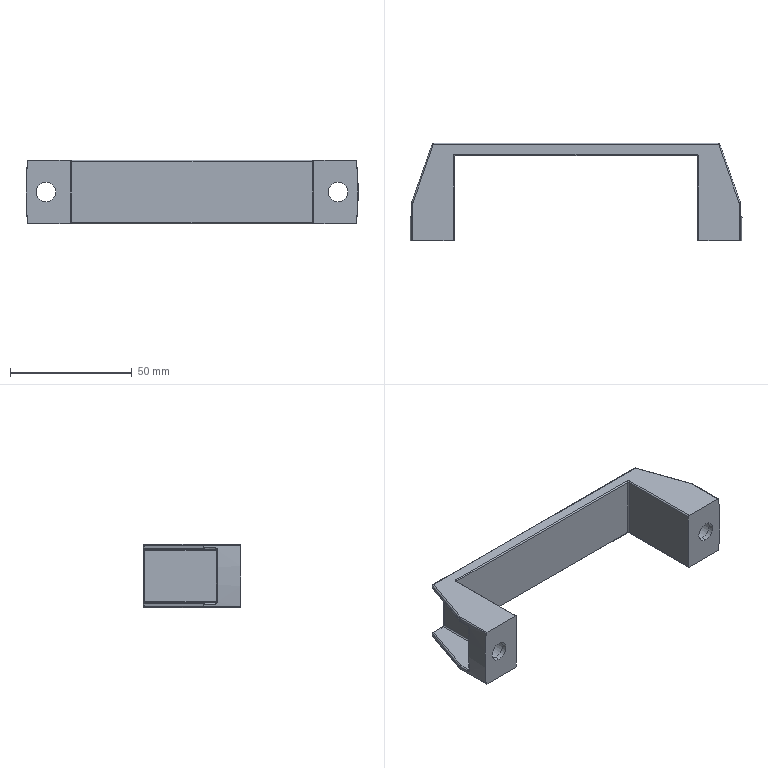Part | SolidWorks | features BaseBody 1 | 1 solid | 110 faces | box 136.5 x 40 x 26 mm | volume 27538 mm3 | cylinder 54 | spline 34 | plane 22 | commonest cylinder face diameters 1 x44 8 x4 10 x4 226.083 x2